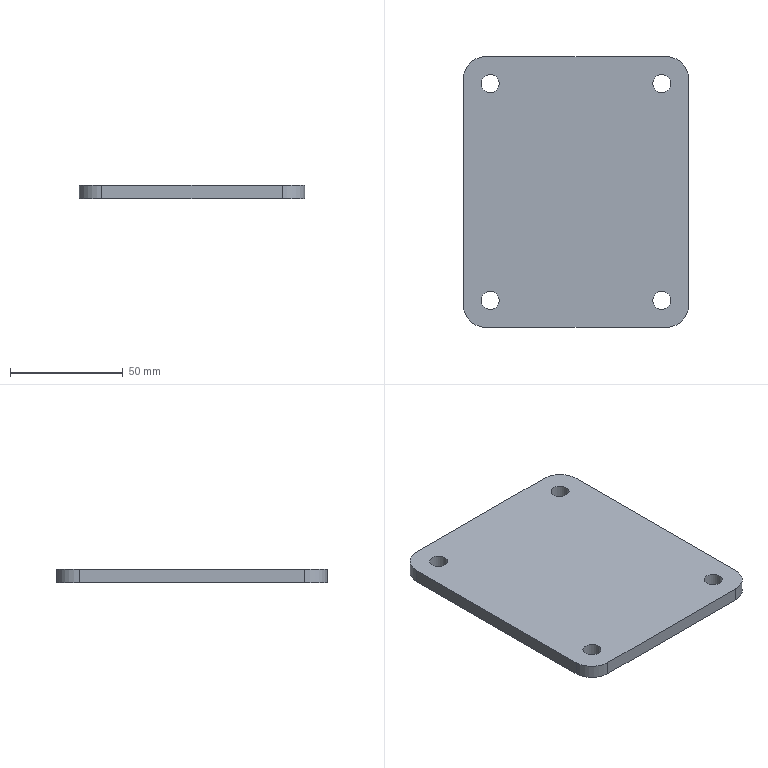Part | NX | features DATUM_CSYS 2, EXTRUDE 1, SKETCH 1 | 1 solid | 14 faces | box 100 x 120 x 6 mm | volume 70279 mm3 | cylinder 8 | plane 6 | commonest cylinder face diameters 8 x4 20 x4
STEP:
#1=CARTESIAN_POINT('',(-50.,50.,0.));
#2=VERTEX_POINT('',#1);
#3=CARTESIAN_POINT('',(-50.,-50.,0.));
#4=VERTEX_POINT('',#3);
#5=CARTESIAN_POINT('',(-50.,50.,0.));
#6=DIRECTION('',(0.,-1.,0.));
#7=VECTOR('',#6,1000.);
#8=LINE('',#5,#7);
#9=EDGE_CURVE('',#2,#4,#8,.T.);
#10=ORIENTED_EDGE('',*,*,#9,.F.);
#11=CARTESIAN_POINT('',(-50.,50.,-6.));
#12=VERTEX_POINT('',#11);
#13=CARTESIAN_POINT('',(-50.,50.,-6.));
#14=DIRECTION('',(0.,0.,1.));
#15=VECTOR('',#14,1000.);
#16=LINE('',#13,#15);
#17=EDGE_CURVE('',#12,#2,#16,.T.);
#18=ORIENTED_EDGE('',*,*,#17,.F.);
#19=CARTESIAN_POINT('',(-50.,-50.,-6.));
#20=VERTEX_POINT('',#19);
#21=CARTESIAN_POINT('',(-50.,50.,-6.));
#22=DIRECTION('',(0.,-1.,0.));
#23=VECTOR('',#22,1000.);
#24=LINE('',#21,#23);
#25=EDGE_CURVE('',#12,#20,#24,.T.);
#26=ORIENTED_EDGE('',*,*,#25,.T.);
#27=CARTESIAN_POINT('',(-50.,-50.,-6.));
#28=DIRECTION('',(0.,0.,1.));
#29=VECTOR('',#28,1000.);
#30=LINE('',#27,#29);
#31=EDGE_CURVE('',#20,#4,#30,.T.);
#32=ORIENTED_EDGE('',*,*,#31,.T.);
#33=EDGE_LOOP('',(#10,#18,#26,#32));
#34=FACE_BOUND('',#33,.T.);
#35=CARTESIAN_POINT('',(-50.,50.,-6.));
#36=DIRECTION('',(-1.,0.,0.));
#37=DIRECTION('',(0.,0.,1.));
#38=AXIS2_PLACEMENT_3D('',#35,#36,#37);
#39=PLANE('',#38);
#40=ADVANCED_FACE('',(#34),#39,.T.);
#41=CARTESIAN_POINT('',(-40.,-60.,0.));
#42=VERTEX_POINT('',#41);
#43=CARTESIAN_POINT('',(-40.,-50.,0.));
#44=DIRECTION('',(0.,0.,1.));
#45=DIRECTION('',(0.,-1.,0.));
#46=AXIS2_PLACEMENT_3D('',#43,#44,#45);
#47=CIRCLE('',#46,10.);
#48=EDGE_CURVE('',#4,#42,#47,.T.);
#49=ORIENTED_EDGE('',*,*,#48,.F.);
#50=ORIENTED_EDGE('',*,*,#31,.F.);
#51=CARTESIAN_POINT('',(-40.,-60.,-6.));
#52=VERTEX_POINT('',#51);
#53=CARTESIAN_POINT('',(-40.,-50.,-6.));
#54=DIRECTION('',(0.,0.,1.));
#55=DIRECTION('',(0.,-1.,0.));
#56=AXIS2_PLACEMENT_3D('',#53,#54,#55);
#57=CIRCLE('',#56,10.);
#58=EDGE_CURVE('',#20,#52,#57,.T.);
#59=ORIENTED_EDGE('',*,*,#58,.T.);
#60=CARTESIAN_POINT('',(-40.,-60.,-6.));
#61=DIRECTION('',(0.,0.,1.));
#62=VECTOR('',#61,1000.);
#63=LINE('',#60,#62);
#64=EDGE_CURVE('',#52,#42,#63,.T.);
#65=ORIENTED_EDGE('',*,*,#64,.T.);
#66=EDGE_LOOP('',(#49,#50,#59,#65));
#67=FACE_BOUND('',#66,.T.);
#68=CARTESIAN_POINT('',(-40.,-50.,-6.));
#69=DIRECTION('',(0.,0.,1.));
#70=DIRECTION('',(1.,0.,0.));
#71=AXIS2_PLACEMENT_3D('',#68,#69,#70);
#72=CYLINDRICAL_SURFACE('',#71,10.);
#73=ADVANCED_FACE('',(#67),#72,.T.);
#74=CARTESIAN_POINT('',(40.,-60.,0.));
#75=VERTEX_POINT('',#74);
#76=CARTESIAN_POINT('',(-40.,-60.,0.));
#77=DIRECTION('',(1.,0.,0.));
#78=VECTOR('',#77,1000.);
#79=LINE('',#76,#78);
#80=EDGE_CURVE('',#42,#75,#79,.T.);
#81=ORIENTED_EDGE('',*,*,#80,.F.);
#82=ORIENTED_EDGE('',*,*,#64,.F.);
#83=CARTESIAN_POINT('',(40.,-60.,-6.));
#84=VERTEX_POINT('',#83);
#85=CARTESIAN_POINT('',(-40.,-60.,-6.));
#86=DIRECTION('',(1.,0.,0.));
#87=VECTOR('',#86,1000.);
#88=LINE('',#85,#87);
#89=EDGE_CURVE('',#52,#84,#88,.T.);
#90=ORIENTED_EDGE('',*,*,#89,.T.);
#91=CARTESIAN_POINT('',(40.,-60.,-6.));
#92=DIRECTION('',(0.,0.,1.));
#93=VECTOR('',#92,1000.);
#94=LINE('',#91,#93);
#95=EDGE_CURVE('',#84,#75,#94,.T.);
#96=ORIENTED_EDGE('',*,*,#95,.T.);
#97=EDGE_LOOP('',(#81,#82,#90,#96));
#98=FACE_BOUND('',#97,.T.);
#99=CARTESIAN_POINT('',(-40.,-60.,-6.));
#100=DIRECTION('',(0.,-1.,0.));
#101=DIRECTION('',(0.,0.,-1.));
#102=AXIS2_PLACEMENT_3D('',#99,#100,#101);
#103=PLANE('',#102);
#104=ADVANCED_FACE('',(#98),#103,.T.);
#105=CARTESIAN_POINT('',(50.,-50.,0.));
#106=VERTEX_POINT('',#105);
#107=CARTESIAN_POINT('',(40.,-50.,0.));
#108=DIRECTION('',(0.,0.,1.));
#109=DIRECTION('',(0.,-1.,0.));
#110=AXIS2_PLACEMENT_3D('',#107,#108,#109);
#111=CIRCLE('',#110,10.);
#112=EDGE_CURVE('',#75,#106,#111,.T.);
#113=ORIENTED_EDGE('',*,*,#112,.F.);
#114=ORIENTED_EDGE('',*,*,#95,.F.);
#115=CARTESIAN_POINT('',(50.,-50.,-6.));
#116=VERTEX_POINT('',#115);
#117=CARTESIAN_POINT('',(40.,-50.,-6.));
#118=DIRECTION('',(0.,0.,1.));
#119=DIRECTION('',(0.,-1.,0.));
#120=AXIS2_PLACEMENT_3D('',#117,#118,#119);
#121=CIRCLE('',#120,10.);
#122=EDGE_CURVE('',#84,#116,#121,.T.);
#123=ORIENTED_EDGE('',*,*,#122,.T.);
#124=CARTESIAN_POINT('',(50.,-50.,-6.));
#125=DIRECTION('',(0.,0.,1.));
#126=VECTOR('',#125,1000.);
#127=LINE('',#124,#126);
#128=EDGE_CURVE('',#116,#106,#127,.T.);
#129=ORIENTED_EDGE('',*,*,#128,.T.);
#130=EDGE_LOOP('',(#113,#114,#123,#129));
#131=FACE_BOUND('',#130,.T.);
#132=CARTESIAN_POINT('',(40.,-50.,-6.));
#133=DIRECTION('',(0.,0.,1.));
#134=DIRECTION('',(1.,0.,0.));
#135=AXIS2_PLACEMENT_3D('',#132,#133,#134);
#136=CYLINDRICAL_SURFACE('',#135,10.);
#137=ADVANCED_FACE('',(#131),#136,.T.);
#138=CARTESIAN_POINT('',(50.,50.,0.));
#139=VERTEX_POINT('',#138);
#140=CARTESIAN_POINT('',(50.,-50.,0.));
#141=DIRECTION('',(0.,1.,0.));
#142=VECTOR('',#141,1000.);
#143=LINE('',#140,#142);
#144=EDGE_CURVE('',#106,#139,#143,.T.);
#145=ORIENTED_EDGE('',*,*,#144,.F.);
#146=ORIENTED_EDGE('',*,*,#128,.F.);
#147=CARTESIAN_POINT('',(50.,50.,-6.));
#148=VERTEX_POINT('',#147);
#149=CARTESIAN_POINT('',(50.,-50.,-6.));
#150=DIRECTION('',(0.,1.,0.));
#151=VECTOR('',#150,1000.);
#152=LINE('',#149,#151);
#153=EDGE_CURVE('',#116,#148,#152,.T.);
#154=ORIENTED_EDGE('',*,*,#153,.T.);
#155=CARTESIAN_POINT('',(50.,50.,-6.));
#156=DIRECTION('',(0.,0.,1.));
#157=VECTOR('',#156,1000.);
#158=LINE('',#155,#157);
#159=EDGE_CURVE('',#148,#139,#158,.T.);
#160=ORIENTED_EDGE('',*,*,#159,.T.);
#161=EDGE_LOOP('',(#145,#146,#154,#160));
#162=FACE_BOUND('',#161,.T.);
#163=CARTESIAN_POINT('',(50.,-50.,-6.));
#164=DIRECTION('',(1.,0.,0.));
#165=DIRECTION('',(0.,0.,-1.));
#166=AXIS2_PLACEMENT_3D('',#163,#164,#165);
#167=PLANE('',#166);
#168=ADVANCED_FACE('',(#162),#167,.T.);
#169=CARTESIAN_POINT('',(40.,60.,0.));
#170=VERTEX_POINT('',#169);
#171=CARTESIAN_POINT('',(40.,50.,0.));
#172=DIRECTION('',(0.,0.,1.));
#173=DIRECTION('',(0.,-1.,0.));
#174=AXIS2_PLACEMENT_3D('',#171,#172,#173);
#175=CIRCLE('',#174,10.);
#176=EDGE_CURVE('',#139,#170,#175,.T.);
#177=ORIENTED_EDGE('',*,*,#176,.F.);
#178=ORIENTED_EDGE('',*,*,#159,.F.);
#179=CARTESIAN_POINT('',(40.,60.,-6.));
#180=VERTEX_POINT('',#179);
#181=CARTESIAN_POINT('',(40.,50.,-6.));
#182=DIRECTION('',(0.,0.,1.));
#183=DIRECTION('',(0.,-1.,0.));
#184=AXIS2_PLACEMENT_3D('',#181,#182,#183);
#185=CIRCLE('',#184,10.);
#186=EDGE_CURVE('',#148,#180,#185,.T.);
#187=ORIENTED_EDGE('',*,*,#186,.T.);
#188=CARTESIAN_POINT('',(40.,60.,-6.));
#189=DIRECTION('',(0.,0.,1.));
#190=VECTOR('',#189,1000.);
#191=LINE('',#188,#190);
#192=EDGE_CURVE('',#180,#170,#191,.T.);
#193=ORIENTED_EDGE('',*,*,#192,.T.);
#194=EDGE_LOOP('',(#177,#178,#187,#193));
#195=FACE_BOUND('',#194,.T.);
#196=CARTESIAN_POINT('',(40.,50.,-6.));
#197=DIRECTION('',(0.,0.,1.));
#198=DIRECTION('',(1.,0.,0.));
#199=AXIS2_PLACEMENT_3D('',#196,#197,#198);
#200=CYLINDRICAL_SURFACE('',#199,10.);
#201=ADVANCED_FACE('',(#195),#200,.T.);
#202=CARTESIAN_POINT('',(-40.,60.,0.));
#203=VERTEX_POINT('',#202);
#204=CARTESIAN_POINT('',(40.,60.,0.));
#205=DIRECTION('',(-1.,0.,0.));
#206=VECTOR('',#205,1000.);
#207=LINE('',#204,#206);
#208=EDGE_CURVE('',#170,#203,#207,.T.);
#209=ORIENTED_EDGE('',*,*,#208,.F.);
#210=ORIENTED_EDGE('',*,*,#192,.F.);
#211=CARTESIAN_POINT('',(-40.,60.,-6.));
#212=VERTEX_POINT('',#211);
#213=CARTESIAN_POINT('',(40.,60.,-6.));
#214=DIRECTION('',(-1.,0.,0.));
#215=VECTOR('',#214,1000.);
#216=LINE('',#213,#215);
#217=EDGE_CURVE('',#180,#212,#216,.T.);
#218=ORIENTED_EDGE('',*,*,#217,.T.);
#219=CARTESIAN_POINT('',(-40.,60.,-6.));
#220=DIRECTION('',(0.,0.,1.));
#221=VECTOR('',#220,1000.);
#222=LINE('',#219,#221);
#223=EDGE_CURVE('',#212,#203,#222,.T.);
#224=ORIENTED_EDGE('',*,*,#223,.T.);
#225=EDGE_LOOP('',(#209,#210,#218,#224));
#226=FACE_BOUND('',#225,.T.);
#227=CARTESIAN_POINT('',(40.,60.,-6.));
#228=DIRECTION('',(0.,1.,0.));
#229=DIRECTION('',(0.,0.,1.));
#230=AXIS2_PLACEMENT_3D('',#227,#228,#229);
#231=PLANE('',#230);
#232=ADVANCED_FACE('',(#226),#231,.T.);
#233=CARTESIAN_POINT('',(-38.,44.,-6.));
#234=VERTEX_POINT('',#233);
#235=CARTESIAN_POINT('',(-38.,48.,-6.));
#236=DIRECTION('',(0.,0.,1.));
#237=DIRECTION('',(0.,-1.,0.));
#238=AXIS2_PLACEMENT_3D('',#235,#236,#237);
#239=CIRCLE('',#238,4.);
#240=EDGE_CURVE('',#234,#234,#239,.T.);
#241=ORIENTED_EDGE('',*,*,#240,.F.);
#242=EDGE_LOOP('',(#241));
#243=FACE_BOUND('',#242,.T.);
#244=CARTESIAN_POINT('',(-38.,44.,0.));
#245=VERTEX_POINT('',#244);
#246=CARTESIAN_POINT('',(-38.,48.,0.));
#247=DIRECTION('',(0.,0.,1.));
#248=DIRECTION('',(0.,-1.,0.));
#249=AXIS2_PLACEMENT_3D('',#246,#247,#248);
#250=CIRCLE('',#249,4.);
#251=EDGE_CURVE('',#245,#245,#250,.T.);
#252=ORIENTED_EDGE('',*,*,#251,.T.);
#253=EDGE_LOOP('',(#252));
#254=FACE_BOUND('',#253,.T.);
#255=CARTESIAN_POINT('',(-38.,48.,-6.));
#256=DIRECTION('',(0.,0.,1.));
#257=DIRECTION('',(1.,0.,0.));
#258=AXIS2_PLACEMENT_3D('',#255,#256,#257);
#259=CYLINDRICAL_SURFACE('',#258,4.);
#260=ADVANCED_FACE('',(#243,#254),#259,.F.);
#261=CARTESIAN_POINT('',(38.,-44.,-6.));
#262=VERTEX_POINT('',#261);
#263=CARTESIAN_POINT('',(38.,-48.,-6.));
#264=DIRECTION('',(0.,0.,1.));
#265=DIRECTION('',(0.,1.,0.));
#266=AXIS2_PLACEMENT_3D('',#263,#264,#265);
#267=CIRCLE('',#266,4.);
#268=EDGE_CURVE('',#262,#262,#267,.T.);
#269=ORIENTED_EDGE('',*,*,#268,.F.);
#270=EDGE_LOOP('',(#269));
#271=FACE_BOUND('',#270,.T.);
#272=CARTESIAN_POINT('',(38.,-44.,0.));
#273=VERTEX_POINT('',#272);
#274=CARTESIAN_POINT('',(38.,-48.,0.));
#275=DIRECTION('',(0.,0.,1.));
#276=DIRECTION('',(0.,1.,0.));
#277=AXIS2_PLACEMENT_3D('',#274,#275,#276);
#278=CIRCLE('',#277,4.);
#279=EDGE_CURVE('',#273,#273,#278,.T.);
#280=ORIENTED_EDGE('',*,*,#279,.T.);
#281=EDGE_LOOP('',(#280));
#282=FACE_BOUND('',#281,.T.);
#283=CARTESIAN_POINT('',(38.,-48.,-6.));
#284=DIRECTION('',(0.,0.,1.));
#285=DIRECTION('',(1.,0.,0.));
#286=AXIS2_PLACEMENT_3D('',#283,#284,#285);
#287=CYLINDRICAL_SURFACE('',#286,4.);
#288=ADVANCED_FACE('',(#271,#282),#287,.F.);
#289=CARTESIAN_POINT('',(38.,44.,-6.));
#290=VERTEX_POINT('',#289);
#291=CARTESIAN_POINT('',(38.,48.,-6.));
#292=DIRECTION('',(0.,0.,-1.));
#293=DIRECTION('',(0.,-1.,0.));
#294=AXIS2_PLACEMENT_3D('',#291,#292,#293);
#295=CIRCLE('',#294,4.);
#296=EDGE_CURVE('',#290,#290,#295,.T.);
#297=ORIENTED_EDGE('',*,*,#296,.T.);
#298=EDGE_LOOP('',(#297));
#299=FACE_BOUND('',#298,.T.);
#300=CARTESIAN_POINT('',(38.,44.,0.));
#301=VERTEX_POINT('',#300);
#302=CARTESIAN_POINT('',(38.,48.,0.));
#303=DIRECTION('',(0.,0.,-1.));
#304=DIRECTION('',(0.,-1.,0.));
#305=AXIS2_PLACEMENT_3D('',#302,#303,#304);
#306=CIRCLE('',#305,4.);
#307=EDGE_CURVE('',#301,#301,#306,.T.);
#308=ORIENTED_EDGE('',*,*,#307,.F.);
#309=EDGE_LOOP('',(#308));
#310=FACE_BOUND('',#309,.T.);
#311=CARTESIAN_POINT('',(38.,48.,-6.));
#312=DIRECTION('',(0.,0.,1.));
#313=DIRECTION('',(1.,0.,0.));
#314=AXIS2_PLACEMENT_3D('',#311,#312,#313);
#315=CYLINDRICAL_SURFACE('',#314,4.);
#316=ADVANCED_FACE('',(#299,#310),#315,.F.);
#317=CARTESIAN_POINT('',(-40.,50.,0.));
#318=DIRECTION('',(0.,0.,1.));
#319=DIRECTION('',(0.,-1.,0.));
#320=AXIS2_PLACEMENT_3D('',#317,#318,#319);
#321=CIRCLE('',#320,10.);
#322=EDGE_CURVE('',#203,#2,#321,.T.);
#323=ORIENTED_EDGE('',*,*,#322,.F.);
#324=ORIENTED_EDGE('',*,*,#223,.F.);
#325=CARTESIAN_POINT('',(-40.,50.,-6.));
#326=DIRECTION('',(0.,0.,1.));
#327=DIRECTION('',(0.,-1.,0.));
#328=AXIS2_PLACEMENT_3D('',#325,#326,#327);
#329=CIRCLE('',#328,10.);
#330=EDGE_CURVE('',#212,#12,#329,.T.);
#331=ORIENTED_EDGE('',*,*,#330,.T.);
#332=ORIENTED_EDGE('',*,*,#17,.T.);
#333=EDGE_LOOP('',(#323,#324,#331,#332));
#334=FACE_BOUND('',#333,.T.);
#335=CARTESIAN_POINT('',(-40.,50.,-6.));
#336=DIRECTION('',(0.,0.,1.));
#337=DIRECTION('',(1.,0.,0.));
#338=AXIS2_PLACEMENT_3D('',#335,#336,#337);
#339=CYLINDRICAL_SURFACE('',#338,10.);
#340=ADVANCED_FACE('',(#334),#339,.T.);
#341=CARTESIAN_POINT('',(-38.,-44.,-6.));
#342=VERTEX_POINT('',#341);
#343=CARTESIAN_POINT('',(-38.,-48.,-6.));
#344=DIRECTION('',(0.,0.,-1.));
#345=DIRECTION('',(0.,1.,0.));
#346=AXIS2_PLACEMENT_3D('',#343,#344,#345);
#347=CIRCLE('',#346,4.);
#348=EDGE_CURVE('',#342,#342,#347,.T.);
#349=ORIENTED_EDGE('',*,*,#348,.T.);
#350=EDGE_LOOP('',(#349));
#351=FACE_BOUND('',#350,.T.);
#352=CARTESIAN_POINT('',(-38.,-44.,0.));
#353=VERTEX_POINT('',#352);
#354=CARTESIAN_POINT('',(-38.,-48.,0.));
#355=DIRECTION('',(0.,0.,-1.));
#356=DIRECTION('',(0.,1.,0.));
#357=AXIS2_PLACEMENT_3D('',#354,#355,#356);
#358=CIRCLE('',#357,4.);
#359=EDGE_CURVE('',#353,#353,#358,.T.);
#360=ORIENTED_EDGE('',*,*,#359,.F.);
#361=EDGE_LOOP('',(#360));
#362=FACE_BOUND('',#361,.T.);
#363=CARTESIAN_POINT('',(-38.,-48.,-6.));
#364=DIRECTION('',(0.,0.,1.));
#365=DIRECTION('',(1.,0.,0.));
#366=AXIS2_PLACEMENT_3D('',#363,#364,#365);
#367=CYLINDRICAL_SURFACE('',#366,4.);
#368=ADVANCED_FACE('',(#351,#362),#367,.F.);
#369=ORIENTED_EDGE('',*,*,#25,.F.);
#370=ORIENTED_EDGE('',*,*,#330,.F.);
#371=ORIENTED_EDGE('',*,*,#217,.F.);
#372=ORIENTED_EDGE('',*,*,#186,.F.);
#373=ORIENTED_EDGE('',*,*,#153,.F.);
#374=ORIENTED_EDGE('',*,*,#122,.F.);
#375=ORIENTED_EDGE('',*,*,#89,.F.);
#376=ORIENTED_EDGE('',*,*,#58,.F.);
#377=EDGE_LOOP('',(#369,#370,#371,#372,#373,#374,#375,#376));
#378=FACE_BOUND('',#377,.T.);
#379=ORIENTED_EDGE('',*,*,#296,.F.);
#380=EDGE_LOOP('',(#379));
#381=FACE_BOUND('',#380,.T.);
#382=ORIENTED_EDGE('',*,*,#268,.T.);
#383=EDGE_LOOP('',(#382));
#384=FACE_BOUND('',#383,.T.);
#385=ORIENTED_EDGE('',*,*,#240,.T.);
#386=EDGE_LOOP('',(#385));
#387=FACE_BOUND('',#386,.T.);
#388=ORIENTED_EDGE('',*,*,#348,.F.);
#389=EDGE_LOOP('',(#388));
#390=FACE_BOUND('',#389,.T.);
#391=CARTESIAN_POINT('',(-40.,-50.,-6.));
#392=DIRECTION('',(0.,0.,1.));
#393=DIRECTION('',(1.,0.,0.));
#394=AXIS2_PLACEMENT_3D('',#391,#392,#393);
#395=PLANE('',#394);
#396=ADVANCED_FACE('',(#378,#381,#384,#387,#390),#395,.F.);
#397=ORIENTED_EDGE('',*,*,#9,.T.);
#398=ORIENTED_EDGE('',*,*,#48,.T.);
#399=ORIENTED_EDGE('',*,*,#80,.T.);
#400=ORIENTED_EDGE('',*,*,#112,.T.);
#401=ORIENTED_EDGE('',*,*,#144,.T.);
#402=ORIENTED_EDGE('',*,*,#176,.T.);
#403=ORIENTED_EDGE('',*,*,#208,.T.);
#404=ORIENTED_EDGE('',*,*,#322,.T.);
#405=EDGE_LOOP('',(#397,#398,#399,#400,#401,#402,#403,#404));
#406=FACE_BOUND('',#405,.T.);
#407=ORIENTED_EDGE('',*,*,#307,.T.);
#408=EDGE_LOOP('',(#407));
#409=FACE_BOUND('',#408,.T.);
#410=ORIENTED_EDGE('',*,*,#279,.F.);
#411=EDGE_LOOP('',(#410));
#412=FACE_BOUND('',#411,.T.);
#413=ORIENTED_EDGE('',*,*,#251,.F.);
#414=EDGE_LOOP('',(#413));
#415=FACE_BOUND('',#414,.T.);
#416=ORIENTED_EDGE('',*,*,#359,.T.);
#417=EDGE_LOOP('',(#416));
#418=FACE_BOUND('',#417,.T.);
#419=CARTESIAN_POINT('',(-40.,-50.,0.));
#420=DIRECTION('',(0.,0.,1.));
#421=DIRECTION('',(1.,0.,0.));
#422=AXIS2_PLACEMENT_3D('',#419,#420,#421);
#423=PLANE('',#422);
#424=ADVANCED_FACE('',(#406,#409,#412,#415,#418),#423,.T.);
#425=CLOSED_SHELL('',(#40,#73,#104,#137,#168,#201,#232,#260,#288,#316,#340,#368,#396,#424));
#426=MANIFOLD_SOLID_BREP('',#425);
#427=(LENGTH_UNIT()NAMED_UNIT(*)SI_UNIT(.MILLI.,.METRE.));
#428=UNCERTAINTY_MEASURE_WITH_UNIT(LENGTH_MEASURE(0.00001),#427,'','');
#429=(NAMED_UNIT(*)PLANE_ANGLE_UNIT()SI_UNIT($,.RADIAN.));
#430=(NAMED_UNIT(*)SI_UNIT($,.STERADIAN.)SOLID_ANGLE_UNIT());
#431=(GEOMETRIC_REPRESENTATION_CONTEXT(3)GLOBAL_UNCERTAINTY_ASSIGNED_CONTEXT((#428))GLOBAL_UNIT_ASSIGNED_CONTEXT((#427,#429,#430))REPRESENTATION_CONTEXT('',''));
#432=ADVANCED_BREP_SHAPE_REPRESENTATION('',(#426),#431);